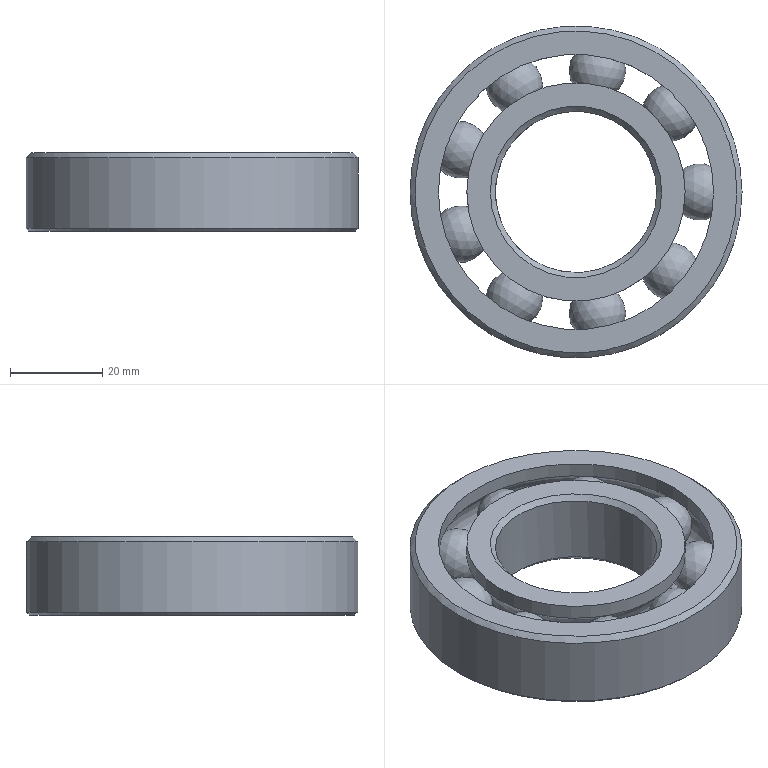Part | NX | 11 solids | 25 faces | box 72 x 72 x 17 mm | volume 35548 mm3 | sphere 9 | cylinder 5 | cone 5 | plane 4 | torus 2 | commonest cylinder face diameters 47.334 x2 35 x1 59.666 x1 72 x1
STEP:
#1=CARTESIAN_POINT('',(-36.,0.,0.6));
#2=VERTEX_POINT('',#1);
#3=CARTESIAN_POINT('',(0.,0.,0.6));
#4=DIRECTION('',(0.,0.,1.));
#5=DIRECTION('',(-1.,0.,0.));
#6=AXIS2_PLACEMENT_3D('',#3,#4,#5);
#7=CIRCLE('',#6,36.);
#8=EDGE_CURVE('',#2,#2,#7,.T.);
#9=ORIENTED_EDGE('',*,*,#8,.T.);
#10=EDGE_LOOP('',(#9));
#11=FACE_BOUND('',#10,.T.);
#12=CARTESIAN_POINT('',(36.,0.,15.9));
#13=VERTEX_POINT('',#12);
#14=CARTESIAN_POINT('',(0.,0.,15.9));
#15=DIRECTION('',(0.,0.,-1.));
#16=DIRECTION('',(1.,0.,0.));
#17=AXIS2_PLACEMENT_3D('',#14,#15,#16);
#18=CIRCLE('',#17,36.);
#19=EDGE_CURVE('',#13,#13,#18,.T.);
#20=ORIENTED_EDGE('',*,*,#19,.T.);
#21=EDGE_LOOP('',(#20));
#22=FACE_BOUND('',#21,.T.);
#23=CARTESIAN_POINT('',(0.,0.,0.));
#24=DIRECTION('',(0.,0.,-1.));
#25=DIRECTION('',(1.,0.,0.));
#26=AXIS2_PLACEMENT_3D('',#23,#24,#25);
#27=CYLINDRICAL_SURFACE('',#26,36.);
#28=ADVANCED_FACE('',(#11,#22),#27,.T.);
#29=CARTESIAN_POINT('',(34.9,0.,17.));
#30=VERTEX_POINT('',#29);
#31=CARTESIAN_POINT('',(0.,0.,17.));
#32=DIRECTION('',(0.,0.,1.));
#33=DIRECTION('',(1.,0.,0.));
#34=AXIS2_PLACEMENT_3D('',#31,#32,#33);
#35=CIRCLE('',#34,34.9);
#36=EDGE_CURVE('',#30,#30,#35,.T.);
#37=ORIENTED_EDGE('',*,*,#36,.T.);
#38=EDGE_LOOP('',(#37));
#39=FACE_BOUND('',#38,.T.);
#40=CARTESIAN_POINT('',(-29.833,0.,17.));
#41=VERTEX_POINT('',#40);
#42=CARTESIAN_POINT('',(0.,0.,17.));
#43=DIRECTION('',(0.,0.,-1.));
#44=DIRECTION('',(-1.,0.,0.));
#45=AXIS2_PLACEMENT_3D('',#42,#43,#44);
#46=CIRCLE('',#45,29.833);
#47=EDGE_CURVE('',#41,#41,#46,.T.);
#48=ORIENTED_EDGE('',*,*,#47,.T.);
#49=EDGE_LOOP('',(#48));
#50=FACE_BOUND('',#49,.T.);
#51=CARTESIAN_POINT('',(36.,0.,17.));
#52=DIRECTION('',(0.,0.,1.));
#53=DIRECTION('',(-1.,0.,0.));
#54=AXIS2_PLACEMENT_3D('',#51,#52,#53);
#55=PLANE('',#54);
#56=ADVANCED_FACE('',(#39,#50),#55,.T.);
#57=CARTESIAN_POINT('',(-29.833,0.,13.84));
#58=VERTEX_POINT('',#57);
#59=CARTESIAN_POINT('',(0.,0.,13.84));
#60=DIRECTION('',(0.,0.,1.));
#61=DIRECTION('',(-1.,0.,0.));
#62=AXIS2_PLACEMENT_3D('',#59,#60,#61);
#63=CIRCLE('',#62,29.833);
#64=EDGE_CURVE('',#58,#58,#63,.T.);
#65=ORIENTED_EDGE('',*,*,#64,.F.);
#66=EDGE_LOOP('',(#65));
#67=FACE_BOUND('',#66,.T.);
#68=ORIENTED_EDGE('',*,*,#47,.F.);
#69=EDGE_LOOP('',(#68));
#70=FACE_BOUND('',#69,.T.);
#71=CARTESIAN_POINT('',(0.,0.,0.));
#72=DIRECTION('',(0.,0.,-1.));
#73=DIRECTION('',(1.,0.,0.));
#74=AXIS2_PLACEMENT_3D('',#71,#72,#73);
#75=CYLINDRICAL_SURFACE('',#74,29.833);
#76=ADVANCED_FACE('',(#67,#70),#75,.F.);
#77=CARTESIAN_POINT('',(-35.4,0.,0.));
#78=VERTEX_POINT('',#77);
#79=CARTESIAN_POINT('',(0.,0.,0.));
#80=DIRECTION('',(0.,0.,-1.));
#81=DIRECTION('',(-1.,0.,0.));
#82=AXIS2_PLACEMENT_3D('',#79,#80,#81);
#83=CIRCLE('',#82,35.4);
#84=EDGE_CURVE('',#78,#78,#83,.T.);
#85=ORIENTED_EDGE('',*,*,#84,.T.);
#86=EDGE_LOOP('',(#85));
#87=FACE_BOUND('',#86,.T.);
#88=CARTESIAN_POINT('',(-31.066,0.,0.));
#89=VERTEX_POINT('',#88);
#90=CARTESIAN_POINT('',(0.,0.,0.));
#91=DIRECTION('',(0.,0.,-1.));
#92=DIRECTION('',(-1.,0.,0.));
#93=AXIS2_PLACEMENT_3D('',#90,#91,#92);
#94=CIRCLE('',#93,31.066);
#95=EDGE_CURVE('',#89,#89,#94,.T.);
#96=ORIENTED_EDGE('',*,*,#95,.F.);
#97=EDGE_LOOP('',(#96));
#98=FACE_BOUND('',#97,.T.);
#99=CARTESIAN_POINT('',(29.833,0.,0.));
#100=DIRECTION('',(0.,0.,-1.));
#101=DIRECTION('',(1.,0.,0.));
#102=AXIS2_PLACEMENT_3D('',#99,#100,#101);
#103=PLANE('',#102);
#104=ADVANCED_FACE('',(#87,#98),#103,.T.);
#105=CARTESIAN_POINT('',(-29.833,0.,3.16));
#106=VERTEX_POINT('',#105);
#107=CARTESIAN_POINT('',(0.,0.,3.16));
#108=DIRECTION('',(0.,0.,-1.));
#109=DIRECTION('',(-1.,0.,0.));
#110=AXIS2_PLACEMENT_3D('',#107,#108,#109);
#111=CIRCLE('',#110,29.833);
#112=EDGE_CURVE('',#106,#106,#111,.T.);
#113=ORIENTED_EDGE('',*,*,#112,.T.);
#114=EDGE_LOOP('',(#113));
#115=FACE_BOUND('',#114,.T.);
#116=ORIENTED_EDGE('',*,*,#64,.T.);
#117=EDGE_LOOP('',(#116));
#118=FACE_BOUND('',#117,.T.);
#119=CARTESIAN_POINT('',(0.,0.,8.5));
#120=DIRECTION('',(0.,0.,-1.));
#121=DIRECTION('',(1.,0.,0.));
#122=AXIS2_PLACEMENT_3D('',#119,#120,#121);
#123=TOROIDAL_SURFACE('',#122,26.75,6.166);
#124=ADVANCED_FACE('',(#115,#118),#123,.F.);
#125=ORIENTED_EDGE('',*,*,#112,.F.);
#126=EDGE_LOOP('',(#125));
#127=FACE_BOUND('',#126,.T.);
#128=ORIENTED_EDGE('',*,*,#95,.T.);
#129=EDGE_LOOP('',(#128));
#130=FACE_BOUND('',#129,.T.);
#131=CARTESIAN_POINT('',(0.,0.,0.));
#132=DIRECTION('',(0.,0.,-1.));
#133=DIRECTION('',(1.,0.,0.));
#134=AXIS2_PLACEMENT_3D('',#131,#132,#133);
#135=CONICAL_SURFACE('',#134,31.066,21.318);
#136=ADVANCED_FACE('',(#127,#130),#135,.F.);
#137=ORIENTED_EDGE('',*,*,#36,.F.);
#138=EDGE_LOOP('',(#137));
#139=FACE_BOUND('',#138,.T.);
#140=ORIENTED_EDGE('',*,*,#19,.F.);
#141=EDGE_LOOP('',(#140));
#142=FACE_BOUND('',#141,.T.);
#143=CARTESIAN_POINT('',(0.,0.,15.9));
#144=DIRECTION('',(0.,0.,-1.));
#145=DIRECTION('',(1.,0.,0.));
#146=AXIS2_PLACEMENT_3D('',#143,#144,#145);
#147=CONICAL_SURFACE('',#146,36.,45.);
#148=ADVANCED_FACE('',(#139,#142),#147,.T.);
#149=ORIENTED_EDGE('',*,*,#8,.F.);
#150=EDGE_LOOP('',(#149));
#151=FACE_BOUND('',#150,.T.);
#152=ORIENTED_EDGE('',*,*,#84,.F.);
#153=EDGE_LOOP('',(#152));
#154=FACE_BOUND('',#153,.T.);
#155=CARTESIAN_POINT('',(0.,0.,0.));
#156=DIRECTION('',(0.,0.,1.));
#157=DIRECTION('',(-1.,0.,0.));
#158=AXIS2_PLACEMENT_3D('',#155,#156,#157);
#159=CONICAL_SURFACE('',#158,35.4,45.);
#160=ADVANCED_FACE('',(#151,#154),#159,.T.);
#161=CLOSED_SHELL('',(#28,#56,#76,#104,#124,#136,#148,#160));
#162=MANIFOLD_SOLID_BREP('',#161);
#163=CARTESIAN_POINT('',(23.667,0.,3.16));
#164=VERTEX_POINT('',#163);
#165=CARTESIAN_POINT('',(0.,0.,3.16));
#166=DIRECTION('',(0.,0.,1.));
#167=DIRECTION('',(1.,0.,0.));
#168=AXIS2_PLACEMENT_3D('',#165,#166,#167);
#169=CIRCLE('',#168,23.667);
#170=EDGE_CURVE('',#164,#164,#169,.T.);
#171=ORIENTED_EDGE('',*,*,#170,.F.);
#172=EDGE_LOOP('',(#171));
#173=FACE_BOUND('',#172,.T.);
#174=CARTESIAN_POINT('',(-23.667,0.,0.));
#175=VERTEX_POINT('',#174);
#176=CARTESIAN_POINT('',(0.,0.,0.));
#177=DIRECTION('',(0.,0.,-1.));
#178=DIRECTION('',(-1.,0.,0.));
#179=AXIS2_PLACEMENT_3D('',#176,#177,#178);
#180=CIRCLE('',#179,23.667);
#181=EDGE_CURVE('',#175,#175,#180,.T.);
#182=ORIENTED_EDGE('',*,*,#181,.F.);
#183=EDGE_LOOP('',(#182));
#184=FACE_BOUND('',#183,.T.);
#185=CARTESIAN_POINT('',(0.,0.,0.));
#186=DIRECTION('',(0.,0.,-1.));
#187=DIRECTION('',(1.,0.,0.));
#188=AXIS2_PLACEMENT_3D('',#185,#186,#187);
#189=CYLINDRICAL_SURFACE('',#188,23.667);
#190=ADVANCED_FACE('',(#173,#184),#189,.T.);
#191=CARTESIAN_POINT('',(-17.5,0.,1.1));
#192=VERTEX_POINT('',#191);
#193=CARTESIAN_POINT('',(0.,0.,1.1));
#194=DIRECTION('',(0.,0.,-1.));
#195=DIRECTION('',(-1.,0.,0.));
#196=AXIS2_PLACEMENT_3D('',#193,#194,#195);
#197=CIRCLE('',#196,17.5);
#198=EDGE_CURVE('',#192,#192,#197,.T.);
#199=ORIENTED_EDGE('',*,*,#198,.T.);
#200=EDGE_LOOP('',(#199));
#201=FACE_BOUND('',#200,.T.);
#202=CARTESIAN_POINT('',(17.5,0.,15.9));
#203=VERTEX_POINT('',#202);
#204=CARTESIAN_POINT('',(0.,0.,15.9));
#205=DIRECTION('',(0.,0.,1.));
#206=DIRECTION('',(1.,0.,0.));
#207=AXIS2_PLACEMENT_3D('',#204,#205,#206);
#208=CIRCLE('',#207,17.5);
#209=EDGE_CURVE('',#203,#203,#208,.T.);
#210=ORIENTED_EDGE('',*,*,#209,.T.);
#211=EDGE_LOOP('',(#210));
#212=FACE_BOUND('',#211,.T.);
#213=CARTESIAN_POINT('',(0.,0.,0.));
#214=DIRECTION('',(0.,0.,-1.));
#215=DIRECTION('',(1.,0.,0.));
#216=AXIS2_PLACEMENT_3D('',#213,#214,#215);
#217=CYLINDRICAL_SURFACE('',#216,17.5);
#218=ADVANCED_FACE('',(#201,#212),#217,.F.);
#219=CARTESIAN_POINT('',(-18.6,0.,0.));
#220=VERTEX_POINT('',#219);
#221=CARTESIAN_POINT('',(0.,0.,0.));
#222=DIRECTION('',(0.,0.,1.));
#223=DIRECTION('',(-1.,0.,0.));
#224=AXIS2_PLACEMENT_3D('',#221,#222,#223);
#225=CIRCLE('',#224,18.6);
#226=EDGE_CURVE('',#220,#220,#225,.T.);
#227=ORIENTED_EDGE('',*,*,#226,.T.);
#228=EDGE_LOOP('',(#227));
#229=FACE_BOUND('',#228,.T.);
#230=ORIENTED_EDGE('',*,*,#181,.T.);
#231=EDGE_LOOP('',(#230));
#232=FACE_BOUND('',#231,.T.);
#233=CARTESIAN_POINT('',(17.5,0.,0.));
#234=DIRECTION('',(0.,0.,-1.));
#235=DIRECTION('',(1.,0.,0.));
#236=AXIS2_PLACEMENT_3D('',#233,#234,#235);
#237=PLANE('',#236);
#238=ADVANCED_FACE('',(#229,#232),#237,.T.);
#239=CARTESIAN_POINT('',(-23.667,0.,13.84));
#240=VERTEX_POINT('',#239);
#241=CARTESIAN_POINT('',(0.,0.,13.84));
#242=DIRECTION('',(0.,0.,-1.));
#243=DIRECTION('',(-1.,0.,0.));
#244=AXIS2_PLACEMENT_3D('',#241,#242,#243);
#245=CIRCLE('',#244,23.667);
#246=EDGE_CURVE('',#240,#240,#245,.T.);
#247=ORIENTED_EDGE('',*,*,#246,.F.);
#248=EDGE_LOOP('',(#247));
#249=FACE_BOUND('',#248,.T.);
#250=CARTESIAN_POINT('',(-23.667,0.,17.));
#251=VERTEX_POINT('',#250);
#252=CARTESIAN_POINT('',(0.,0.,17.));
#253=DIRECTION('',(0.,0.,-1.));
#254=DIRECTION('',(-1.,0.,0.));
#255=AXIS2_PLACEMENT_3D('',#252,#253,#254);
#256=CIRCLE('',#255,23.667);
#257=EDGE_CURVE('',#251,#251,#256,.T.);
#258=ORIENTED_EDGE('',*,*,#257,.T.);
#259=EDGE_LOOP('',(#258));
#260=FACE_BOUND('',#259,.T.);
#261=CARTESIAN_POINT('',(0.,0.,0.));
#262=DIRECTION('',(0.,0.,-1.));
#263=DIRECTION('',(1.,0.,0.));
#264=AXIS2_PLACEMENT_3D('',#261,#262,#263);
#265=CYLINDRICAL_SURFACE('',#264,23.667);
#266=ADVANCED_FACE('',(#249,#260),#265,.T.);
#267=CARTESIAN_POINT('',(18.6,0.,17.));
#268=VERTEX_POINT('',#267);
#269=CARTESIAN_POINT('',(0.,0.,17.));
#270=DIRECTION('',(0.,0.,-1.));
#271=DIRECTION('',(1.,0.,0.));
#272=AXIS2_PLACEMENT_3D('',#269,#270,#271);
#273=CIRCLE('',#272,18.6);
#274=EDGE_CURVE('',#268,#268,#273,.T.);
#275=ORIENTED_EDGE('',*,*,#274,.T.);
#276=EDGE_LOOP('',(#275));
#277=FACE_BOUND('',#276,.T.);
#278=ORIENTED_EDGE('',*,*,#257,.F.);
#279=EDGE_LOOP('',(#278));
#280=FACE_BOUND('',#279,.T.);
#281=CARTESIAN_POINT('',(23.667,0.,17.));
#282=DIRECTION('',(0.,0.,1.));
#283=DIRECTION('',(-1.,0.,0.));
#284=AXIS2_PLACEMENT_3D('',#281,#282,#283);
#285=PLANE('',#284);
#286=ADVANCED_FACE('',(#277,#280),#285,.T.);
#287=ORIENTED_EDGE('',*,*,#170,.T.);
#288=EDGE_LOOP('',(#287));
#289=FACE_BOUND('',#288,.T.);
#290=ORIENTED_EDGE('',*,*,#246,.T.);
#291=EDGE_LOOP('',(#290));
#292=FACE_BOUND('',#291,.T.);
#293=CARTESIAN_POINT('',(0.,0.,8.5));
#294=DIRECTION('',(0.,0.,-1.));
#295=DIRECTION('',(1.,0.,0.));
#296=AXIS2_PLACEMENT_3D('',#293,#294,#295);
#297=TOROIDAL_SURFACE('',#296,26.75,6.166);
#298=ADVANCED_FACE('',(#289,#292),#297,.F.);
#299=ORIENTED_EDGE('',*,*,#226,.F.);
#300=EDGE_LOOP('',(#299));
#301=FACE_BOUND('',#300,.T.);
#302=ORIENTED_EDGE('',*,*,#198,.F.);
#303=EDGE_LOOP('',(#302));
#304=FACE_BOUND('',#303,.T.);
#305=CARTESIAN_POINT('',(0.,0.,1.1));
#306=DIRECTION('',(0.,0.,-1.));
#307=DIRECTION('',(1.,0.,0.));
#308=AXIS2_PLACEMENT_3D('',#305,#306,#307);
#309=CONICAL_SURFACE('',#308,17.5,45.);
#310=ADVANCED_FACE('',(#301,#304),#309,.F.);
#311=ORIENTED_EDGE('',*,*,#209,.F.);
#312=EDGE_LOOP('',(#311));
#313=FACE_BOUND('',#312,.T.);
#314=ORIENTED_EDGE('',*,*,#274,.F.);
#315=EDGE_LOOP('',(#314));
#316=FACE_BOUND('',#315,.T.);
#317=CARTESIAN_POINT('',(0.,0.,17.));
#318=DIRECTION('',(0.,0.,1.));
#319=DIRECTION('',(-1.,0.,0.));
#320=AXIS2_PLACEMENT_3D('',#317,#318,#319);
#321=CONICAL_SURFACE('',#320,18.6,45.);
#322=ADVANCED_FACE('',(#313,#316),#321,.F.);
#323=CLOSED_SHELL('',(#190,#218,#238,#266,#286,#298,#310,#322));
#324=MANIFOLD_SOLID_BREP('',#323);
#325=CARTESIAN_POINT('',(20.492,17.195,2.334));
#326=VERTEX_POINT('',#325);
#327=VERTEX_LOOP('',#326);
#328=FACE_BOUND('',#327,.T.);
#329=CARTESIAN_POINT('',(20.492,17.195,8.5));
#330=DIRECTION('',(0.766,0.6428,0.));
#331=DIRECTION('',(0.,0.,-1.));
#332=AXIS2_PLACEMENT_3D('',#329,#330,#331);
#333=SPHERICAL_SURFACE('',#332,6.166);
#334=ADVANCED_FACE('',(#328),#333,.T.);
#335=CLOSED_SHELL('',(#334));
#336=MANIFOLD_SOLID_BREP('',#335);
#337=CARTESIAN_POINT('',(-25.137,-9.149,2.334));
#338=VERTEX_POINT('',#337);
#339=VERTEX_LOOP('',#338);
#340=FACE_BOUND('',#339,.T.);
#341=CARTESIAN_POINT('',(-25.137,-9.149,8.5));
#342=DIRECTION('',(-0.9397,-0.342,0.));
#343=DIRECTION('',(0.,0.,-1.));
#344=AXIS2_PLACEMENT_3D('',#341,#342,#343);
#345=SPHERICAL_SURFACE('',#344,6.166);
#346=ADVANCED_FACE('',(#340),#345,.T.);
#347=CLOSED_SHELL('',(#346));
#348=MANIFOLD_SOLID_BREP('',#347);
#349=CARTESIAN_POINT('',(4.645,-26.344,2.334));
#350=VERTEX_POINT('',#349);
#351=VERTEX_LOOP('',#350);
#352=FACE_BOUND('',#351,.T.);
#353=CARTESIAN_POINT('',(4.645,-26.344,8.5));
#354=DIRECTION('',(0.1736,-0.9848,0.));
#355=DIRECTION('',(0.,0.,-1.));
#356=AXIS2_PLACEMENT_3D('',#353,#354,#355);
#357=SPHERICAL_SURFACE('',#356,6.166);
#358=ADVANCED_FACE('',(#352),#357,.T.);
#359=CLOSED_SHELL('',(#358));
#360=MANIFOLD_SOLID_BREP('',#359);
#361=CARTESIAN_POINT('',(-25.137,9.149,2.334));
#362=VERTEX_POINT('',#361);
#363=VERTEX_LOOP('',#362);
#364=FACE_BOUND('',#363,.T.);
#365=CARTESIAN_POINT('',(-25.137,9.149,8.5));
#366=DIRECTION('',(-0.9397,0.342,0.));
#367=DIRECTION('',(0.,0.,-1.));
#368=AXIS2_PLACEMENT_3D('',#365,#366,#367);
#369=SPHERICAL_SURFACE('',#368,6.166);
#370=ADVANCED_FACE('',(#364),#369,.T.);
#371=CLOSED_SHELL('',(#370));
#372=MANIFOLD_SOLID_BREP('',#371);
#373=CARTESIAN_POINT('',(-13.375,23.166,2.334));
#374=VERTEX_POINT('',#373);
#375=VERTEX_LOOP('',#374);
#376=FACE_BOUND('',#375,.T.);
#377=CARTESIAN_POINT('',(-13.375,23.166,8.5));
#378=DIRECTION('',(-0.5,0.866,0.));
#379=DIRECTION('',(0.,0.,-1.));
#380=AXIS2_PLACEMENT_3D('',#377,#378,#379);
#381=SPHERICAL_SURFACE('',#380,6.166);
#382=ADVANCED_FACE('',(#376),#381,.T.);
#383=CLOSED_SHELL('',(#382));
#384=MANIFOLD_SOLID_BREP('',#383);
#385=CARTESIAN_POINT('',(20.492,-17.195,2.334));
#386=VERTEX_POINT('',#385);
#387=VERTEX_LOOP('',#386);
#388=FACE_BOUND('',#387,.T.);
#389=CARTESIAN_POINT('',(20.492,-17.195,8.5));
#390=DIRECTION('',(0.766,-0.6428,0.));
#391=DIRECTION('',(0.,0.,-1.));
#392=AXIS2_PLACEMENT_3D('',#389,#390,#391);
#393=SPHERICAL_SURFACE('',#392,6.166);
#394=ADVANCED_FACE('',(#388),#393,.T.);
#395=CLOSED_SHELL('',(#394));
#396=MANIFOLD_SOLID_BREP('',#395);
#397=CARTESIAN_POINT('',(-13.375,-23.166,2.334));
#398=VERTEX_POINT('',#397);
#399=VERTEX_LOOP('',#398);
#400=FACE_BOUND('',#399,.T.);
#401=CARTESIAN_POINT('',(-13.375,-23.166,8.5));
#402=DIRECTION('',(-0.5,-0.866,0.));
#403=DIRECTION('',(0.,0.,-1.));
#404=AXIS2_PLACEMENT_3D('',#401,#402,#403);
#405=SPHERICAL_SURFACE('',#404,6.166);
#406=ADVANCED_FACE('',(#400),#405,.T.);
#407=CLOSED_SHELL('',(#406));
#408=MANIFOLD_SOLID_BREP('',#407);
#409=CARTESIAN_POINT('',(26.75,0.,2.334));
#410=VERTEX_POINT('',#409);
#411=VERTEX_LOOP('',#410);
#412=FACE_BOUND('',#411,.T.);
#413=CARTESIAN_POINT('',(26.75,0.,8.5));
#414=DIRECTION('',(1.,0.,0.));
#415=DIRECTION('',(0.,0.,-1.));
#416=AXIS2_PLACEMENT_3D('',#413,#414,#415);
#417=SPHERICAL_SURFACE('',#416,6.166);
#418=ADVANCED_FACE('',(#412),#417,.T.);
#419=CLOSED_SHELL('',(#418));
#420=MANIFOLD_SOLID_BREP('',#419);
#421=CARTESIAN_POINT('',(4.645,26.344,2.334));
#422=VERTEX_POINT('',#421);
#423=VERTEX_LOOP('',#422);
#424=FACE_BOUND('',#423,.T.);
#425=CARTESIAN_POINT('',(4.645,26.344,8.5));
#426=DIRECTION('',(0.1736,0.9848,0.));
#427=DIRECTION('',(0.,0.,-1.));
#428=AXIS2_PLACEMENT_3D('',#425,#426,#427);
#429=SPHERICAL_SURFACE('',#428,6.166);
#430=ADVANCED_FACE('',(#424),#429,.T.);
#431=CLOSED_SHELL('',(#430));
#432=MANIFOLD_SOLID_BREP('',#431);
#433=(LENGTH_UNIT()NAMED_UNIT(*)SI_UNIT(.MILLI.,.METRE.));
#434=UNCERTAINTY_MEASURE_WITH_UNIT(LENGTH_MEASURE(0.00002),#433,'','');
#435=(NAMED_UNIT(*)PLANE_ANGLE_UNIT()SI_UNIT($,.RADIAN.));
#436=PLANE_ANGLE_MEASURE_WITH_UNIT(PLANE_ANGLE_MEASURE(0.01745),#435);
#437=DIMENSIONAL_EXPONENTS(0.,0.,0.,0.,0.,0.,0.);
#438=(CONVERSION_BASED_UNIT('DEGREE',#436)NAMED_UNIT(#437)PLANE_ANGLE_UNIT());
#439=(NAMED_UNIT(*)SI_UNIT($,.STERADIAN.)SOLID_ANGLE_UNIT());
#440=(GEOMETRIC_REPRESENTATION_CONTEXT(3)GLOBAL_UNCERTAINTY_ASSIGNED_CONTEXT((#434))GLOBAL_UNIT_ASSIGNED_CONTEXT((#433,#438,#439))REPRESENTATION_CONTEXT('',''));
#441=ADVANCED_BREP_SHAPE_REPRESENTATION('',(#162,#324,#336,#348,#360,#372,#384,#396,#408,#420,#432),#440);